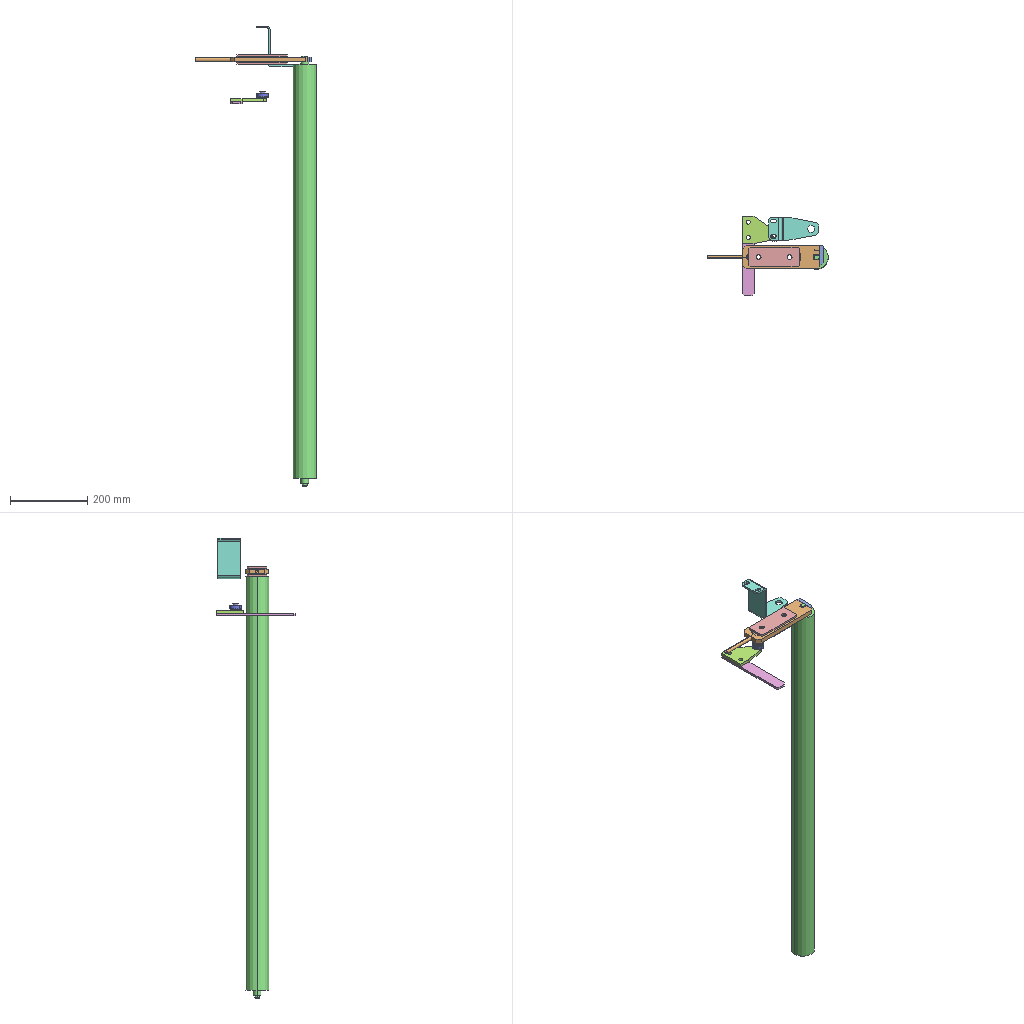Assembly | SolidWorks | 21 different items | 32 placed | box 312 x 205 x 1189 mm
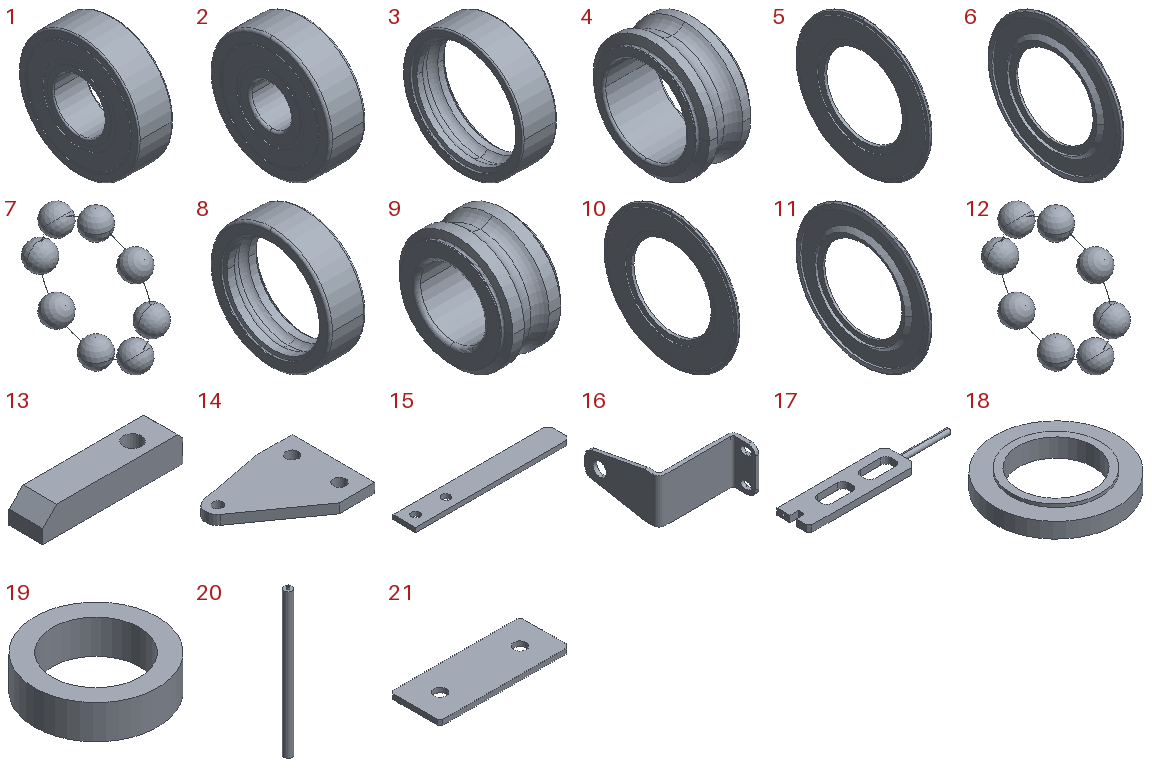Parts list (item | name | quantity | parent item | size | volume | features):
1 | (subassembly) | x2 | - | 8 x 28 x 28 mm | 2775 mm3 | -
2 | (subassembly) | x1 | - | 9 x 30 x 30 mm | 4205 mm3 | -
3 | - | x2 | in 1 | 8 x 28 x 28 mm | 1280 mm3 | features BaseBody 1
4 | - | x2 | in 1 | 8 x 17 x 17 mm | 683.161 mm3 | features BaseBody 1
5 | - | x2 | in 1 | 1.155 x 25.353 x 25.353 mm | 179.548 mm3 | features BaseBody 1
6 | - | x2 | in 1 | 1.155 x 25.353 x 25.353 mm | 179.548 mm3 | features BaseBody 1
7 | - | x2 | in 1 | 4.762 x 24.762 x 24.762 mm | 452.339 mm3 | features BaseBody 1
8 | - | x1 | in 2 | 9 x 30 x 30 mm | 2282 mm3 | features BaseBody 1
9 | - | x1 | in 2 | 9 x 17 x 17 mm | 1119 mm3 | features BaseBody 1
10 | - | x1 | in 2 | 1.155 x 25.353 x 25.353 mm | 176.021 mm3 | features BaseBody 1
11 | - | x1 | in 2 | 1.155 x 25.353 x 25.353 mm | 176.021 mm3 | features BaseBody 1
12 | - | x1 | in 2 | 4.762 x 24.762 x 24.762 mm | 452.339 mm3 | features BaseBody 1
13 | - | x1 | - | 50 x 12 x 10 mm | 5494 mm3 | features Chamfer 1, Extrusion 1, HoleWzd 1
14 | - | x1 | - | 93 x 70 x 8 mm | 35854 mm3 | features Extrusion 1, HoleWzd 1, ICE 1
15 | - | x1 | - | 205 x 30 x 6 mm | 35610 mm3 | features Extrusion 1
16 | - | x1 | - | 105 x 130 x 60 mm | 58783 mm3 | features ICE 4, Fillet 3, Extrusion 1, HoleWzd 1
17 | - | x1 | - | 289.75 x 60 x 12 mm | 104525 mm3 | features Chamfer 3, ICE 3, HoleWzd 2, Extrusion 1, Fillet 1, Revolution 1
18 | - | x4 | - | 20 x 20 x 3 mm | 517.267 mm3 | features Revolution 1
19 | - | x2 | - | 14.5 x 14.5 x 4 mm | 333.669 mm3 | features Revolution 1
20 | - | x1 | - | 60 x 60 x 1111 mm | 3034450 mm3 | features ICE 4, Chamfer 1, Revolution 1
21 | - | x2 | - | 130 x 50 x 5 mm | 31183 mm3 | features Extrusion 1
Mates (type | each side: item.copy, entity, surface, feature):
Concentric | 13.1 face cylinder Ø6.5 (6.5) Diameter Hole1 | 17.1 face cylinder M6 Tapped Hole1
Coincident | 13.1 face plane Boss-Extrude1 | 17.1 face plane Boss-Extrude1
Parallel | 13.1 face plane Boss-Extrude1 | 17.1 face plane Boss-Extrude1
Width | 21.1 face plane Boss-Extrude1 | 21.1 face plane Boss-Extrude1 | 17.1 face plane Boss-Extrude1 | 17.1 face plane Boss-Extrude1
Width | 21.1 face plane Boss-Extrude1 | 21.1 face plane Boss-Extrude1 | 17.1 face plane Cut-Extrude2 | 17.1 face plane Cut-Extrude3
Concentric | 18.1 face cylinder Revolve1 | 18.2 face cylinder Revolve1
Concentric | 4.1 face cylinder 6001-2rsl | 18.2 face cylinder Revolve1
Coincident | 4.1 face plane 6001-2rsl | 18.2 face plane Revolve1
Coincident | 4.1 face plane 6001-2rsl | 18.1 face plane Revolve1
Width | 3.1 face plane 6001-2rsl | 3.1 face plane 6001-2rsl | 17.1 face plane Boss-Extrude1 | 17.1 face plane Boss-Extrude1
Concentric | 21.1 face cylinder Boss-Extrude1 | 4.1 face cylinder 6001-2rsl
Concentric | 18.2 face cylinder Revolve1 | 21.2 face cylinder Boss-Extrude1
Coincident | 18.2 face plane Revolve1 | 21.2 face plane Boss-Extrude1
Coincident | 21.1 edge | 18.1 face plane Revolve1
Coincident | 18.3 face plane Revolve1 | 4.2 face plane 6001-2rsl
Coincident | 4.2 face plane 6001-2rsl | 18.4 face plane Revolve1
Concentric | 3.2 face cylinder 6001-2rsl | 18.4 face cylinder Revolve1
Concentric | 21.1 face cylinder Boss-Extrude1 | 4.2 face cylinder 6001-2rsl
Concentric | 18.3 face cylinder Revolve1 | 4.2 face cylinder 6001-2rsl
Coincident | 21.2 face plane Boss-Extrude1 | 18.3 face plane Revolve1
Concentric | 21.2 face cylinder Boss-Extrude1 | 4.2 face cylinder 6001-2rsl
Concentric | 14.1 face cylinder M10 Tapped Hole1 | 19.1 face cylinder Revolve1
Concentric | 19.1 face cylinder Revolve1 | 8.1 face cylinder 6200-2rsl
Coincident | 19.1 face plane Revolve1 | 9.1 face plane 6200-2rsl
Coincident | 19.2 face plane Revolve1 | 9.1 edge
Concentric | 14.1 face cylinder M10 Tapped Hole1 | 19.2 face cylinder Revolve1
Coincident | 14.1 face plane Boss-Extrude1 | 19.2 face plane Revolve1
Concentric | 14.1 edge | 15.1 face cylinder Boss-Extrude1
Coincident | 14.1 face plane Boss-Extrude1 | 17.1 face plane Boss-Extrude1
Concentric | 14.1 edge | 15.1 edge
Concentric | 14.1 face cylinder Boss-Extrude1 | 15.1 face cylinder Boss-Extrude1
Coincident | 14.1 face plane Boss-Extrude1 | 15.1 face plane Boss-Extrude1
Parallel | 16.1 face plane Boss-Extrude2 | 21.2 face plane Boss-Extrude1
Parallel | 16.1 face plane Boss-Extrude1 | 17.1 face plane Boss-Extrude1
Lock | 21.1 select_type:0 | 15.1 select_type:0
Lock | 16.1 select_type:0 | 17.1 select_type:0
Coincident | 17.1 plane | 20.1 plane
Coincident | 17.1 face plane Cut-Extrude1 | 20.1 face plane Boss-Extrude2
Coincident | 17.1 face plane Boss-Extrude1 | 20.1 face plane Boss-Extrude1